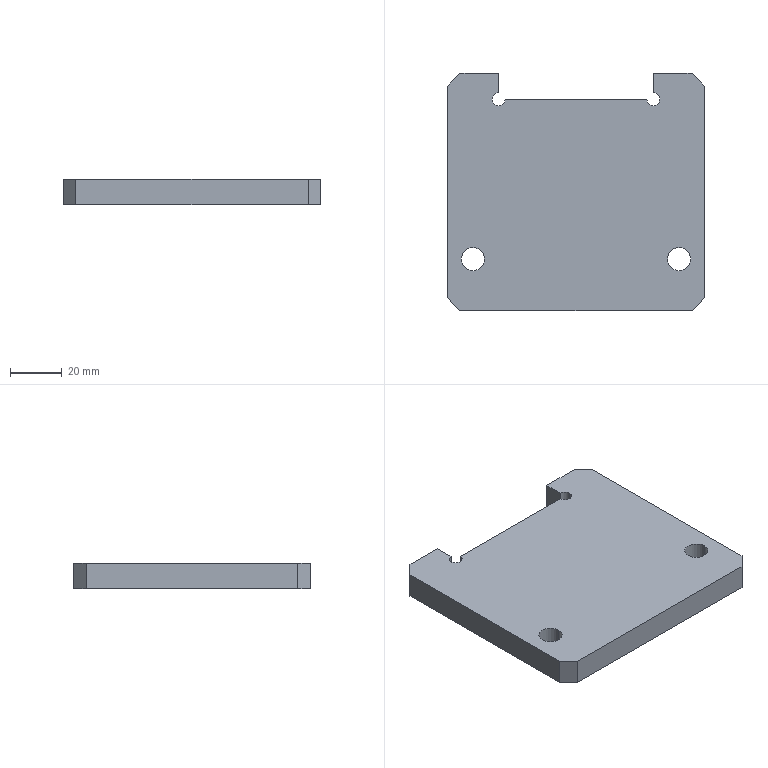Part | SolidWorks | features BaseBody 1 | 1 solid | 29 faces | box 100 x 92 x 10 mm | volume 83534 mm3 | plane 14 | cylinder 11 | cone 4 | commonest cylinder face diameters 4.2 x4 9 x4 5 x3
STEP:
#1=CARTESIAN_POINT('',(35.5,-26.,0.));
#2=VERTEX_POINT('',#1);
#3=CARTESIAN_POINT('',(44.5,-26.,0.));
#4=VERTEX_POINT('',#3);
#5=CARTESIAN_POINT('',(40.,-26.,0.));
#6=DIRECTION('',(0.,0.,1.));
#7=DIRECTION('',(1.,0.,0.));
#8=AXIS2_PLACEMENT_3D('',#5,#6,#7);
#9=CIRCLE('',#8,4.5);
#10=EDGE_CURVE('',#2,#4,#9,.T.);
#11=ORIENTED_EDGE('',*,*,#10,.F.);
#12=CARTESIAN_POINT('',(35.5,-26.,10.));
#13=VERTEX_POINT('',#12);
#14=CARTESIAN_POINT('',(35.5,-26.,10.));
#15=DIRECTION('',(0.,0.,1.));
#16=VECTOR('',#15,1000.);
#17=LINE('',#14,#16);
#18=EDGE_CURVE('',#2,#13,#17,.T.);
#19=ORIENTED_EDGE('',*,*,#18,.T.);
#20=CARTESIAN_POINT('',(44.5,-26.,10.));
#21=VERTEX_POINT('',#20);
#22=CARTESIAN_POINT('',(40.,-26.,10.));
#23=DIRECTION('',(0.,0.,1.));
#24=DIRECTION('',(1.,0.,0.));
#25=AXIS2_PLACEMENT_3D('',#22,#23,#24);
#26=CIRCLE('',#25,4.5);
#27=EDGE_CURVE('',#13,#21,#26,.T.);
#28=ORIENTED_EDGE('',*,*,#27,.T.);
#29=CARTESIAN_POINT('',(44.5,-26.,10.));
#30=DIRECTION('',(0.,0.,1.));
#31=VECTOR('',#30,1000.);
#32=LINE('',#29,#31);
#33=EDGE_CURVE('',#4,#21,#32,.T.);
#34=ORIENTED_EDGE('',*,*,#33,.F.);
#35=EDGE_LOOP('',(#11,#19,#28,#34));
#36=FACE_OUTER_BOUND('',#35,.T.);
#37=CARTESIAN_POINT('',(40.,-26.,10.));
#38=DIRECTION('',(0.,0.,1.));
#39=DIRECTION('',(1.,0.,0.));
#40=AXIS2_PLACEMENT_3D('',#37,#38,#39);
#41=CYLINDRICAL_SURFACE('',#40,4.5);
#42=ADVANCED_FACE('',(#36),#41,.F.);
#43=CARTESIAN_POINT('',(-44.5,-26.,0.));
#44=VERTEX_POINT('',#43);
#45=CARTESIAN_POINT('',(-35.5,-26.,0.));
#46=VERTEX_POINT('',#45);
#47=CARTESIAN_POINT('',(-40.,-26.,0.));
#48=DIRECTION('',(0.,0.,1.));
#49=DIRECTION('',(1.,0.,0.));
#50=AXIS2_PLACEMENT_3D('',#47,#48,#49);
#51=CIRCLE('',#50,4.5);
#52=EDGE_CURVE('',#44,#46,#51,.T.);
#53=ORIENTED_EDGE('',*,*,#52,.F.);
#54=CARTESIAN_POINT('',(-44.5,-26.,10.));
#55=VERTEX_POINT('',#54);
#56=CARTESIAN_POINT('',(-44.5,-26.,10.));
#57=DIRECTION('',(0.,0.,1.));
#58=VECTOR('',#57,1000.);
#59=LINE('',#56,#58);
#60=EDGE_CURVE('',#44,#55,#59,.T.);
#61=ORIENTED_EDGE('',*,*,#60,.T.);
#62=CARTESIAN_POINT('',(-35.5,-26.,10.));
#63=VERTEX_POINT('',#62);
#64=CARTESIAN_POINT('',(-40.,-26.,10.));
#65=DIRECTION('',(0.,0.,1.));
#66=DIRECTION('',(1.,0.,0.));
#67=AXIS2_PLACEMENT_3D('',#64,#65,#66);
#68=CIRCLE('',#67,4.5);
#69=EDGE_CURVE('',#55,#63,#68,.T.);
#70=ORIENTED_EDGE('',*,*,#69,.T.);
#71=CARTESIAN_POINT('',(-35.5,-26.,10.));
#72=DIRECTION('',(0.,0.,1.));
#73=VECTOR('',#72,1000.);
#74=LINE('',#71,#73);
#75=EDGE_CURVE('',#46,#63,#74,.T.);
#76=ORIENTED_EDGE('',*,*,#75,.F.);
#77=EDGE_LOOP('',(#53,#61,#70,#76));
#78=FACE_OUTER_BOUND('',#77,.T.);
#79=CARTESIAN_POINT('',(-40.,-26.,10.));
#80=DIRECTION('',(0.,0.,1.));
#81=DIRECTION('',(1.,0.,0.));
#82=AXIS2_PLACEMENT_3D('',#79,#80,#81);
#83=CYLINDRICAL_SURFACE('',#82,4.5);
#84=ADVANCED_FACE('',(#78),#83,.F.);
#85=CARTESIAN_POINT('',(-20.,22.,2.9));
#86=VERTEX_POINT('',#85);
#87=CARTESIAN_POINT('',(-20.,22.,7.1));
#88=VERTEX_POINT('',#87);
#89=CARTESIAN_POINT('',(-20.,22.,5.));
#90=DIRECTION('',(0.,1.,0.));
#91=DIRECTION('',(0.,0.,1.));
#92=AXIS2_PLACEMENT_3D('',#89,#90,#91);
#93=CIRCLE('',#92,2.1);
#94=EDGE_CURVE('',#86,#88,#93,.T.);
#95=ORIENTED_EDGE('',*,*,#94,.F.);
#96=CARTESIAN_POINT('',(-20.,36.,2.9));
#97=VERTEX_POINT('',#96);
#98=CARTESIAN_POINT('',(-20.,36.,2.9));
#99=DIRECTION('',(0.,1.,0.));
#100=VECTOR('',#99,1000.);
#101=LINE('',#98,#100);
#102=EDGE_CURVE('',#86,#97,#101,.T.);
#103=ORIENTED_EDGE('',*,*,#102,.T.);
#104=CARTESIAN_POINT('',(-20.,36.,7.1));
#105=VERTEX_POINT('',#104);
#106=CARTESIAN_POINT('',(-20.,36.,5.));
#107=DIRECTION('',(0.,1.,0.));
#108=DIRECTION('',(0.,0.,1.));
#109=AXIS2_PLACEMENT_3D('',#106,#107,#108);
#110=CIRCLE('',#109,2.1);
#111=EDGE_CURVE('',#97,#105,#110,.T.);
#112=ORIENTED_EDGE('',*,*,#111,.T.);
#113=CARTESIAN_POINT('',(-20.,36.,7.1));
#114=DIRECTION('',(0.,1.,0.));
#115=VECTOR('',#114,1000.);
#116=LINE('',#113,#115);
#117=EDGE_CURVE('',#88,#105,#116,.T.);
#118=ORIENTED_EDGE('',*,*,#117,.F.);
#119=EDGE_LOOP('',(#95,#103,#112,#118));
#120=FACE_OUTER_BOUND('',#119,.T.);
#121=CARTESIAN_POINT('',(-20.,36.,5.));
#122=DIRECTION('',(0.,1.,0.));
#123=DIRECTION('',(0.,0.,1.));
#124=AXIS2_PLACEMENT_3D('',#121,#122,#123);
#125=CYLINDRICAL_SURFACE('',#124,2.1);
#126=ADVANCED_FACE('',(#120),#125,.F.);
#127=CARTESIAN_POINT('',(-20.,20.738,5.));
#128=VERTEX_POINT('',#127);
#129=CARTESIAN_POINT('',(-20.,22.,7.1));
#130=DIRECTION('',(0.,0.515,0.8572));
#131=VECTOR('',#130,1000.);
#132=LINE('',#129,#131);
#133=EDGE_CURVE('',#128,#88,#132,.T.);
#134=ORIENTED_EDGE('',*,*,#133,.F.);
#135=CARTESIAN_POINT('',(-20.,22.,2.9));
#136=DIRECTION('',(0.,0.515,-0.8572));
#137=VECTOR('',#136,1000.);
#138=LINE('',#135,#137);
#139=EDGE_CURVE('',#128,#86,#138,.T.);
#140=ORIENTED_EDGE('',*,*,#139,.T.);
#141=ORIENTED_EDGE('',*,*,#94,.T.);
#142=EDGE_LOOP('',(#134,#140,#141));
#143=FACE_OUTER_BOUND('',#142,.T.);
#144=CARTESIAN_POINT('',(-20.,22.,5.));
#145=DIRECTION('',(0.,1.,0.));
#146=DIRECTION('',(0.,0.,1.));
#147=AXIS2_PLACEMENT_3D('',#144,#145,#146);
#148=CONICAL_SURFACE('',#147,2.1,1.03);
#149=ADVANCED_FACE('',(#143),#148,.F.);
#150=CARTESIAN_POINT('',(20.,22.,2.9));
#151=VERTEX_POINT('',#150);
#152=CARTESIAN_POINT('',(20.,22.,7.1));
#153=VERTEX_POINT('',#152);
#154=CARTESIAN_POINT('',(20.,22.,5.));
#155=DIRECTION('',(0.,1.,0.));
#156=DIRECTION('',(0.,0.,1.));
#157=AXIS2_PLACEMENT_3D('',#154,#155,#156);
#158=CIRCLE('',#157,2.1);
#159=EDGE_CURVE('',#151,#153,#158,.T.);
#160=ORIENTED_EDGE('',*,*,#159,.F.);
#161=CARTESIAN_POINT('',(20.,36.,2.9));
#162=VERTEX_POINT('',#161);
#163=CARTESIAN_POINT('',(20.,36.,2.9));
#164=DIRECTION('',(0.,1.,0.));
#165=VECTOR('',#164,1000.);
#166=LINE('',#163,#165);
#167=EDGE_CURVE('',#151,#162,#166,.T.);
#168=ORIENTED_EDGE('',*,*,#167,.T.);
#169=CARTESIAN_POINT('',(20.,36.,7.1));
#170=VERTEX_POINT('',#169);
#171=CARTESIAN_POINT('',(20.,36.,5.));
#172=DIRECTION('',(0.,1.,0.));
#173=DIRECTION('',(0.,0.,1.));
#174=AXIS2_PLACEMENT_3D('',#171,#172,#173);
#175=CIRCLE('',#174,2.1);
#176=EDGE_CURVE('',#162,#170,#175,.T.);
#177=ORIENTED_EDGE('',*,*,#176,.T.);
#178=CARTESIAN_POINT('',(20.,36.,7.1));
#179=DIRECTION('',(0.,1.,0.));
#180=VECTOR('',#179,1000.);
#181=LINE('',#178,#180);
#182=EDGE_CURVE('',#153,#170,#181,.T.);
#183=ORIENTED_EDGE('',*,*,#182,.F.);
#184=EDGE_LOOP('',(#160,#168,#177,#183));
#185=FACE_OUTER_BOUND('',#184,.T.);
#186=CARTESIAN_POINT('',(20.,36.,5.));
#187=DIRECTION('',(0.,1.,0.));
#188=DIRECTION('',(0.,0.,1.));
#189=AXIS2_PLACEMENT_3D('',#186,#187,#188);
#190=CYLINDRICAL_SURFACE('',#189,2.1);
#191=ADVANCED_FACE('',(#185),#190,.F.);
#192=CARTESIAN_POINT('',(20.,20.738,5.));
#193=VERTEX_POINT('',#192);
#194=CARTESIAN_POINT('',(20.,22.,7.1));
#195=DIRECTION('',(0.,0.515,0.8572));
#196=VECTOR('',#195,1000.);
#197=LINE('',#194,#196);
#198=EDGE_CURVE('',#193,#153,#197,.T.);
#199=ORIENTED_EDGE('',*,*,#198,.F.);
#200=CARTESIAN_POINT('',(20.,22.,2.9));
#201=DIRECTION('',(0.,0.515,-0.8572));
#202=VECTOR('',#201,1000.);
#203=LINE('',#200,#202);
#204=EDGE_CURVE('',#193,#151,#203,.T.);
#205=ORIENTED_EDGE('',*,*,#204,.T.);
#206=ORIENTED_EDGE('',*,*,#159,.T.);
#207=EDGE_LOOP('',(#199,#205,#206));
#208=FACE_OUTER_BOUND('',#207,.T.);
#209=CARTESIAN_POINT('',(20.,22.,5.));
#210=DIRECTION('',(0.,1.,0.));
#211=DIRECTION('',(0.,0.,1.));
#212=AXIS2_PLACEMENT_3D('',#209,#210,#211);
#213=CONICAL_SURFACE('',#212,2.1,1.03);
#214=ADVANCED_FACE('',(#208),#213,.F.);
#215=CARTESIAN_POINT('',(32.5,36.,0.));
#216=VERTEX_POINT('',#215);
#217=CARTESIAN_POINT('',(30.,38.5,0.));
#218=VERTEX_POINT('',#217);
#219=CARTESIAN_POINT('',(30.,36.,0.));
#220=DIRECTION('',(0.,0.,1.));
#221=DIRECTION('',(1.,0.,0.));
#222=AXIS2_PLACEMENT_3D('',#219,#220,#221);
#223=CIRCLE('',#222,2.5);
#224=EDGE_CURVE('',#216,#218,#223,.T.);
#225=ORIENTED_EDGE('',*,*,#224,.F.);
#226=CARTESIAN_POINT('',(32.5,36.,10.));
#227=VERTEX_POINT('',#226);
#228=CARTESIAN_POINT('',(32.5,36.,0.));
#229=DIRECTION('',(0.,0.,1.));
#230=VECTOR('',#229,1000.);
#231=LINE('',#228,#230);
#232=EDGE_CURVE('',#216,#227,#231,.T.);
#233=ORIENTED_EDGE('',*,*,#232,.T.);
#234=CARTESIAN_POINT('',(30.,38.5,10.));
#235=VERTEX_POINT('',#234);
#236=CARTESIAN_POINT('',(30.,36.,10.));
#237=DIRECTION('',(0.,0.,1.));
#238=DIRECTION('',(1.,0.,0.));
#239=AXIS2_PLACEMENT_3D('',#236,#237,#238);
#240=CIRCLE('',#239,2.5);
#241=EDGE_CURVE('',#227,#235,#240,.T.);
#242=ORIENTED_EDGE('',*,*,#241,.T.);
#243=CARTESIAN_POINT('',(30.,38.5,0.));
#244=DIRECTION('',(0.,0.,1.));
#245=VECTOR('',#244,1000.);
#246=LINE('',#243,#245);
#247=EDGE_CURVE('',#218,#235,#246,.T.);
#248=ORIENTED_EDGE('',*,*,#247,.F.);
#249=EDGE_LOOP('',(#225,#233,#242,#248));
#250=FACE_OUTER_BOUND('',#249,.T.);
#251=CARTESIAN_POINT('',(30.,36.,0.));
#252=DIRECTION('',(0.,0.,1.));
#253=DIRECTION('',(1.,0.,0.));
#254=AXIS2_PLACEMENT_3D('',#251,#252,#253);
#255=CYLINDRICAL_SURFACE('',#254,2.5);
#256=ADVANCED_FACE('',(#250),#255,.F.);
#257=CARTESIAN_POINT('',(-30.,46.,0.));
#258=VERTEX_POINT('',#257);
#259=CARTESIAN_POINT('',(-45.,46.,0.));
#260=VERTEX_POINT('',#259);
#261=CARTESIAN_POINT('',(50.,46.,0.));
#262=DIRECTION('',(-1.,0.,0.));
#263=VECTOR('',#262,1000.);
#264=LINE('',#261,#263);
#265=EDGE_CURVE('',#258,#260,#264,.T.);
#266=ORIENTED_EDGE('',*,*,#265,.T.);
#267=CARTESIAN_POINT('',(-45.,46.,10.));
#268=VERTEX_POINT('',#267);
#269=CARTESIAN_POINT('',(-45.,46.,10.));
#270=DIRECTION('',(0.,0.,1.));
#271=VECTOR('',#270,1000.);
#272=LINE('',#269,#271);
#273=EDGE_CURVE('',#260,#268,#272,.T.);
#274=ORIENTED_EDGE('',*,*,#273,.T.);
#275=CARTESIAN_POINT('',(-30.,46.,10.));
#276=VERTEX_POINT('',#275);
#277=CARTESIAN_POINT('',(50.,46.,10.));
#278=DIRECTION('',(-1.,0.,0.));
#279=VECTOR('',#278,1000.);
#280=LINE('',#277,#279);
#281=EDGE_CURVE('',#276,#268,#280,.T.);
#282=ORIENTED_EDGE('',*,*,#281,.F.);
#283=CARTESIAN_POINT('',(-30.,46.,10.));
#284=DIRECTION('',(0.,0.,-1.));
#285=VECTOR('',#284,1000.);
#286=LINE('',#283,#285);
#287=EDGE_CURVE('',#276,#258,#286,.T.);
#288=ORIENTED_EDGE('',*,*,#287,.T.);
#289=EDGE_LOOP('',(#266,#274,#282,#288));
#290=FACE_OUTER_BOUND('',#289,.T.);
#291=CARTESIAN_POINT('',(50.,46.,10.));
#292=DIRECTION('',(0.,-1.,0.));
#293=DIRECTION('',(1.,0.,0.));
#294=AXIS2_PLACEMENT_3D('',#291,#292,#293);
#295=PLANE('',#294);
#296=ADVANCED_FACE('',(#290),#295,.F.);
#297=CARTESIAN_POINT('',(-50.,41.,0.));
#298=VERTEX_POINT('',#297);
#299=CARTESIAN_POINT('',(-50.,-41.,0.));
#300=VERTEX_POINT('',#299);
#301=CARTESIAN_POINT('',(-50.,-46.,0.));
#302=DIRECTION('',(0.,-1.,0.));
#303=VECTOR('',#302,1000.);
#304=LINE('',#301,#303);
#305=EDGE_CURVE('',#298,#300,#304,.T.);
#306=ORIENTED_EDGE('',*,*,#305,.T.);
#307=CARTESIAN_POINT('',(-50.,-41.,10.));
#308=VERTEX_POINT('',#307);
#309=CARTESIAN_POINT('',(-50.,-41.,10.));
#310=DIRECTION('',(0.,0.,1.));
#311=VECTOR('',#310,1000.);
#312=LINE('',#309,#311);
#313=EDGE_CURVE('',#300,#308,#312,.T.);
#314=ORIENTED_EDGE('',*,*,#313,.T.);
#315=CARTESIAN_POINT('',(-50.,41.,10.));
#316=VERTEX_POINT('',#315);
#317=CARTESIAN_POINT('',(-50.,-46.,10.));
#318=DIRECTION('',(0.,-1.,0.));
#319=VECTOR('',#318,1000.);
#320=LINE('',#317,#319);
#321=EDGE_CURVE('',#316,#308,#320,.T.);
#322=ORIENTED_EDGE('',*,*,#321,.F.);
#323=CARTESIAN_POINT('',(-50.,41.,10.));
#324=DIRECTION('',(0.,0.,-1.));
#325=VECTOR('',#324,1000.);
#326=LINE('',#323,#325);
#327=EDGE_CURVE('',#316,#298,#326,.T.);
#328=ORIENTED_EDGE('',*,*,#327,.T.);
#329=EDGE_LOOP('',(#306,#314,#322,#328));
#330=FACE_OUTER_BOUND('',#329,.T.);
#331=CARTESIAN_POINT('',(-50.,-46.,10.));
#332=DIRECTION('',(1.,0.,0.));
#333=DIRECTION('',(0.,0.,-1.));
#334=AXIS2_PLACEMENT_3D('',#331,#332,#333);
#335=PLANE('',#334);
#336=ADVANCED_FACE('',(#330),#335,.F.);
#337=CARTESIAN_POINT('',(-45.,-46.,10.));
#338=VERTEX_POINT('',#337);
#339=CARTESIAN_POINT('',(45.,-46.,10.));
#340=VERTEX_POINT('',#339);
#341=CARTESIAN_POINT('',(50.,-46.,10.));
#342=DIRECTION('',(1.,0.,0.));
#343=VECTOR('',#342,1000.);
#344=LINE('',#341,#343);
#345=EDGE_CURVE('',#338,#340,#344,.T.);
#346=ORIENTED_EDGE('',*,*,#345,.F.);
#347=CARTESIAN_POINT('',(-45.,-46.,0.));
#348=VERTEX_POINT('',#347);
#349=CARTESIAN_POINT('',(-45.,-46.,10.));
#350=DIRECTION('',(0.,0.,-1.));
#351=VECTOR('',#350,1000.);
#352=LINE('',#349,#351);
#353=EDGE_CURVE('',#338,#348,#352,.T.);
#354=ORIENTED_EDGE('',*,*,#353,.T.);
#355=CARTESIAN_POINT('',(45.,-46.,0.));
#356=VERTEX_POINT('',#355);
#357=CARTESIAN_POINT('',(50.,-46.,0.));
#358=DIRECTION('',(1.,0.,0.));
#359=VECTOR('',#358,1000.);
#360=LINE('',#357,#359);
#361=EDGE_CURVE('',#348,#356,#360,.T.);
#362=ORIENTED_EDGE('',*,*,#361,.T.);
#363=CARTESIAN_POINT('',(45.,-46.,10.));
#364=DIRECTION('',(0.,0.,1.));
#365=VECTOR('',#364,1000.);
#366=LINE('',#363,#365);
#367=EDGE_CURVE('',#356,#340,#366,.T.);
#368=ORIENTED_EDGE('',*,*,#367,.T.);
#369=EDGE_LOOP('',(#346,#354,#362,#368));
#370=FACE_OUTER_BOUND('',#369,.T.);
#371=CARTESIAN_POINT('',(50.,-46.,10.));
#372=DIRECTION('',(0.,1.,0.));
#373=DIRECTION('',(-1.,0.,0.));
#374=AXIS2_PLACEMENT_3D('',#371,#372,#373);
#375=PLANE('',#374);
#376=ADVANCED_FACE('',(#370),#375,.F.);
#377=CARTESIAN_POINT('',(50.,-41.,10.));
#378=VERTEX_POINT('',#377);
#379=CARTESIAN_POINT('',(50.,41.,10.));
#380=VERTEX_POINT('',#379);
#381=CARTESIAN_POINT('',(50.,-46.,10.));
#382=DIRECTION('',(0.,1.,0.));
#383=VECTOR('',#382,1000.);
#384=LINE('',#381,#383);
#385=EDGE_CURVE('',#378,#380,#384,.T.);
#386=ORIENTED_EDGE('',*,*,#385,.F.);
#387=CARTESIAN_POINT('',(50.,-41.,0.));
#388=VERTEX_POINT('',#387);
#389=CARTESIAN_POINT('',(50.,-41.,10.));
#390=DIRECTION('',(0.,0.,-1.));
#391=VECTOR('',#390,1000.);
#392=LINE('',#389,#391);
#393=EDGE_CURVE('',#378,#388,#392,.T.);
#394=ORIENTED_EDGE('',*,*,#393,.T.);
#395=CARTESIAN_POINT('',(50.,41.,0.));
#396=VERTEX_POINT('',#395);
#397=CARTESIAN_POINT('',(50.,-46.,0.));
#398=DIRECTION('',(0.,1.,0.));
#399=VECTOR('',#398,1000.);
#400=LINE('',#397,#399);
#401=EDGE_CURVE('',#388,#396,#400,.T.);
#402=ORIENTED_EDGE('',*,*,#401,.T.);
#403=CARTESIAN_POINT('',(50.,41.,10.));
#404=DIRECTION('',(0.,0.,1.));
#405=VECTOR('',#404,1000.);
#406=LINE('',#403,#405);
#407=EDGE_CURVE('',#396,#380,#406,.T.);
#408=ORIENTED_EDGE('',*,*,#407,.T.);
#409=EDGE_LOOP('',(#386,#394,#402,#408));
#410=FACE_OUTER_BOUND('',#409,.T.);
#411=CARTESIAN_POINT('',(50.,-46.,10.));
#412=DIRECTION('',(-1.,0.,0.));
#413=DIRECTION('',(0.,0.,1.));
#414=AXIS2_PLACEMENT_3D('',#411,#412,#413);
#415=PLANE('',#414);
#416=ADVANCED_FACE('',(#410),#415,.F.);
#417=CARTESIAN_POINT('',(45.,46.,10.));
#418=VERTEX_POINT('',#417);
#419=CARTESIAN_POINT('',(30.,46.,10.));
#420=VERTEX_POINT('',#419);
#421=CARTESIAN_POINT('',(50.,46.,10.));
#422=DIRECTION('',(-1.,0.,0.));
#423=VECTOR('',#422,1000.);
#424=LINE('',#421,#423);
#425=EDGE_CURVE('',#418,#420,#424,.T.);
#426=ORIENTED_EDGE('',*,*,#425,.F.);
#427=CARTESIAN_POINT('',(45.,46.,0.));
#428=VERTEX_POINT('',#427);
#429=CARTESIAN_POINT('',(45.,46.,10.));
#430=DIRECTION('',(0.,0.,-1.));
#431=VECTOR('',#430,1000.);
#432=LINE('',#429,#431);
#433=EDGE_CURVE('',#418,#428,#432,.T.);
#434=ORIENTED_EDGE('',*,*,#433,.T.);
#435=CARTESIAN_POINT('',(30.,46.,0.));
#436=VERTEX_POINT('',#435);
#437=CARTESIAN_POINT('',(50.,46.,0.));
#438=DIRECTION('',(-1.,0.,0.));
#439=VECTOR('',#438,1000.);
#440=LINE('',#437,#439);
#441=EDGE_CURVE('',#428,#436,#440,.T.);
#442=ORIENTED_EDGE('',*,*,#441,.T.);
#443=CARTESIAN_POINT('',(30.,46.,10.));
#444=DIRECTION('',(0.,0.,1.));
#445=VECTOR('',#444,1000.);
#446=LINE('',#443,#445);
#447=EDGE_CURVE('',#436,#420,#446,.T.);
#448=ORIENTED_EDGE('',*,*,#447,.T.);
#449=EDGE_LOOP('',(#426,#434,#442,#448));
#450=FACE_OUTER_BOUND('',#449,.T.);
#451=CARTESIAN_POINT('',(50.,46.,10.));
#452=DIRECTION('',(0.,-1.,0.));
#453=DIRECTION('',(1.,0.,0.));
#454=AXIS2_PLACEMENT_3D('',#451,#452,#453);
#455=PLANE('',#454);
#456=ADVANCED_FACE('',(#450),#455,.F.);
#457=CARTESIAN_POINT('',(40.,-26.,10.));
#458=DIRECTION('',(0.,0.,1.));
#459=DIRECTION('',(1.,0.,0.));
#460=AXIS2_PLACEMENT_3D('',#457,#458,#459);
#461=CIRCLE('',#460,4.5);
#462=EDGE_CURVE('',#21,#13,#461,.T.);
#463=ORIENTED_EDGE('',*,*,#462,.F.);
#464=ORIENTED_EDGE('',*,*,#27,.F.);
#465=EDGE_LOOP('',(#463,#464));
#466=FACE_BOUND('',#465,.T.);
#467=CARTESIAN_POINT('',(-40.,-26.,10.));
#468=DIRECTION('',(0.,0.,1.));
#469=DIRECTION('',(1.,0.,0.));
#470=AXIS2_PLACEMENT_3D('',#467,#468,#469);
#471=CIRCLE('',#470,4.5);
#472=EDGE_CURVE('',#63,#55,#471,.T.);
#473=ORIENTED_EDGE('',*,*,#472,.F.);
#474=ORIENTED_EDGE('',*,*,#69,.F.);
#475=EDGE_LOOP('',(#473,#474));
#476=FACE_BOUND('',#475,.T.);
#477=CARTESIAN_POINT('',(27.5,36.,10.));
#478=VERTEX_POINT('',#477);
#479=CARTESIAN_POINT('',(30.,36.,10.));
#480=DIRECTION('',(0.,0.,1.));
#481=DIRECTION('',(1.,0.,0.));
#482=AXIS2_PLACEMENT_3D('',#479,#480,#481);
#483=CIRCLE('',#482,2.5);
#484=EDGE_CURVE('',#478,#227,#483,.T.);
#485=ORIENTED_EDGE('',*,*,#484,.F.);
#486=CARTESIAN_POINT('',(-27.5,36.,10.));
#487=VERTEX_POINT('',#486);
#488=CARTESIAN_POINT('',(30.,36.,10.));
#489=DIRECTION('',(1.,0.,0.));
#490=VECTOR('',#489,1000.);
#491=LINE('',#488,#490);
#492=EDGE_CURVE('',#487,#478,#491,.T.);
#493=ORIENTED_EDGE('',*,*,#492,.F.);
#494=CARTESIAN_POINT('',(-30.,38.5,10.));
#495=VERTEX_POINT('',#494);
#496=CARTESIAN_POINT('',(-30.,36.,10.));
#497=DIRECTION('',(0.,0.,1.));
#498=DIRECTION('',(1.,0.,0.));
#499=AXIS2_PLACEMENT_3D('',#496,#497,#498);
#500=CIRCLE('',#499,2.5);
#501=EDGE_CURVE('',#495,#487,#500,.T.);
#502=ORIENTED_EDGE('',*,*,#501,.F.);
#503=CARTESIAN_POINT('',(-30.,56.,10.));
#504=DIRECTION('',(0.,-1.,0.));
#505=VECTOR('',#504,1000.);
#506=LINE('',#503,#505);
#507=EDGE_CURVE('',#276,#495,#506,.T.);
#508=ORIENTED_EDGE('',*,*,#507,.F.);
#509=ORIENTED_EDGE('',*,*,#281,.T.);
#510=CARTESIAN_POINT('',(-45.5,45.5,10.));
#511=DIRECTION('',(-0.7071,-0.7071,0.));
#512=VECTOR('',#511,1000.);
#513=LINE('',#510,#512);
#514=EDGE_CURVE('',#268,#316,#513,.T.);
#515=ORIENTED_EDGE('',*,*,#514,.T.);
#516=ORIENTED_EDGE('',*,*,#321,.T.);
#517=CARTESIAN_POINT('',(-45.5,-45.5,10.));
#518=DIRECTION('',(0.7071,-0.7071,0.));
#519=VECTOR('',#518,1000.);
#520=LINE('',#517,#519);
#521=EDGE_CURVE('',#308,#338,#520,.T.);
#522=ORIENTED_EDGE('',*,*,#521,.T.);
#523=ORIENTED_EDGE('',*,*,#345,.T.);
#524=CARTESIAN_POINT('',(45.5,-45.5,10.));
#525=DIRECTION('',(0.7071,0.7071,0.));
#526=VECTOR('',#525,1000.);
#527=LINE('',#524,#526);
#528=EDGE_CURVE('',#340,#378,#527,.T.);
#529=ORIENTED_EDGE('',*,*,#528,.T.);
#530=ORIENTED_EDGE('',*,*,#385,.T.);
#531=CARTESIAN_POINT('',(45.5,45.5,10.));
#532=DIRECTION('',(-0.7071,0.7071,0.));
#533=VECTOR('',#532,1000.);
#534=LINE('',#531,#533);
#535=EDGE_CURVE('',#380,#418,#534,.T.);
#536=ORIENTED_EDGE('',*,*,#535,.T.);
#537=ORIENTED_EDGE('',*,*,#425,.T.);
#538=CARTESIAN_POINT('',(30.,56.,10.));
#539=DIRECTION('',(0.,1.,0.));
#540=VECTOR('',#539,1000.);
#541=LINE('',#538,#540);
#542=EDGE_CURVE('',#235,#420,#541,.T.);
#543=ORIENTED_EDGE('',*,*,#542,.F.);
#544=ORIENTED_EDGE('',*,*,#241,.F.);
#545=EDGE_LOOP('',(#485,#493,#502,#508,#509,#515,#516,#522,#523,#529,#530,#536,#537,#543,#544));
#546=FACE_OUTER_BOUND('',#545,.T.);
#547=CARTESIAN_POINT('',(0.,0.,10.));
#548=DIRECTION('',(0.,0.,1.));
#549=DIRECTION('',(1.,0.,0.));
#550=AXIS2_PLACEMENT_3D('',#547,#548,#549);
#551=PLANE('',#550);
#552=ADVANCED_FACE('',(#466,#476,#546),#551,.T.);
#553=CARTESIAN_POINT('',(40.,-26.,0.));
#554=DIRECTION('',(0.,0.,1.));
#555=DIRECTION('',(1.,0.,0.));
#556=AXIS2_PLACEMENT_3D('',#553,#554,#555);
#557=CIRCLE('',#556,4.5);
#558=EDGE_CURVE('',#4,#2,#557,.T.);
#559=ORIENTED_EDGE('',*,*,#558,.T.);
#560=ORIENTED_EDGE('',*,*,#10,.T.);
#561=EDGE_LOOP('',(#559,#560));
#562=FACE_BOUND('',#561,.T.);
#563=CARTESIAN_POINT('',(-40.,-26.,0.));
#564=DIRECTION('',(0.,0.,1.));
#565=DIRECTION('',(1.,0.,0.));
#566=AXIS2_PLACEMENT_3D('',#563,#564,#565);
#567=CIRCLE('',#566,4.5);
#568=EDGE_CURVE('',#46,#44,#567,.T.);
#569=ORIENTED_EDGE('',*,*,#568,.T.);
#570=ORIENTED_EDGE('',*,*,#52,.T.);
#571=EDGE_LOOP('',(#569,#570));
#572=FACE_BOUND('',#571,.T.);
#573=CARTESIAN_POINT('',(-27.5,36.,0.));
#574=VERTEX_POINT('',#573);
#575=CARTESIAN_POINT('',(27.5,36.,0.));
#576=VERTEX_POINT('',#575);
#577=CARTESIAN_POINT('',(30.,36.,0.));
#578=DIRECTION('',(1.,0.,0.));
#579=VECTOR('',#578,1000.);
#580=LINE('',#577,#579);
#581=EDGE_CURVE('',#574,#576,#580,.T.);
#582=ORIENTED_EDGE('',*,*,#581,.T.);
#583=CARTESIAN_POINT('',(30.,36.,0.));
#584=DIRECTION('',(0.,0.,1.));
#585=DIRECTION('',(1.,0.,0.));
#586=AXIS2_PLACEMENT_3D('',#583,#584,#585);
#587=CIRCLE('',#586,2.5);
#588=EDGE_CURVE('',#576,#216,#587,.T.);
#589=ORIENTED_EDGE('',*,*,#588,.T.);
#590=ORIENTED_EDGE('',*,*,#224,.T.);
#591=CARTESIAN_POINT('',(30.,56.,0.));
#592=DIRECTION('',(0.,1.,0.));
#593=VECTOR('',#592,1000.);
#594=LINE('',#591,#593);
#595=EDGE_CURVE('',#218,#436,#594,.T.);
#596=ORIENTED_EDGE('',*,*,#595,.T.);
#597=ORIENTED_EDGE('',*,*,#441,.F.);
#598=CARTESIAN_POINT('',(45.,46.,0.));
#599=DIRECTION('',(0.7071,-0.7071,0.));
#600=VECTOR('',#599,1000.);
#601=LINE('',#598,#600);
#602=EDGE_CURVE('',#428,#396,#601,.T.);
#603=ORIENTED_EDGE('',*,*,#602,.T.);
#604=ORIENTED_EDGE('',*,*,#401,.F.);
#605=CARTESIAN_POINT('',(50.,-41.,0.));
#606=DIRECTION('',(-0.7071,-0.7071,0.));
#607=VECTOR('',#606,1000.);
#608=LINE('',#605,#607);
#609=EDGE_CURVE('',#388,#356,#608,.T.);
#610=ORIENTED_EDGE('',*,*,#609,.T.);
#611=ORIENTED_EDGE('',*,*,#361,.F.);
#612=CARTESIAN_POINT('',(-45.,-46.,0.));
#613=DIRECTION('',(-0.7071,0.7071,0.));
#614=VECTOR('',#613,1000.);
#615=LINE('',#612,#614);
#616=EDGE_CURVE('',#348,#300,#615,.T.);
#617=ORIENTED_EDGE('',*,*,#616,.T.);
#618=ORIENTED_EDGE('',*,*,#305,.F.);
#619=CARTESIAN_POINT('',(-50.,41.,0.));
#620=DIRECTION('',(0.7071,0.7071,0.));
#621=VECTOR('',#620,1000.);
#622=LINE('',#619,#621);
#623=EDGE_CURVE('',#298,#260,#622,.T.);
#624=ORIENTED_EDGE('',*,*,#623,.T.);
#625=ORIENTED_EDGE('',*,*,#265,.F.);
#626=CARTESIAN_POINT('',(-30.,38.5,0.));
#627=VERTEX_POINT('',#626);
#628=CARTESIAN_POINT('',(-30.,0.,0.));
#629=DIRECTION('',(0.,-1.,0.));
#630=VECTOR('',#629,1000.);
#631=LINE('',#628,#630);
#632=EDGE_CURVE('',#258,#627,#631,.T.);
#633=ORIENTED_EDGE('',*,*,#632,.T.);
#634=CARTESIAN_POINT('',(-30.,36.,0.));
#635=DIRECTION('',(0.,0.,1.));
#636=DIRECTION('',(1.,0.,0.));
#637=AXIS2_PLACEMENT_3D('',#634,#635,#636);
#638=CIRCLE('',#637,2.5);
#639=EDGE_CURVE('',#627,#574,#638,.T.);
#640=ORIENTED_EDGE('',*,*,#639,.T.);
#641=EDGE_LOOP('',(#582,#589,#590,#596,#597,#603,#604,#610,#611,#617,#618,#624,#625,#633,#640));
#642=FACE_OUTER_BOUND('',#641,.T.);
#643=CARTESIAN_POINT('',(0.,0.,0.));
#644=DIRECTION('',(0.,0.,1.));
#645=DIRECTION('',(1.,0.,0.));
#646=AXIS2_PLACEMENT_3D('',#643,#644,#645);
#647=PLANE('',#646);
#648=ADVANCED_FACE('',(#562,#572,#642),#647,.F.);
#649=ORIENTED_EDGE('',*,*,#507,.T.);
#650=CARTESIAN_POINT('',(-30.,38.5,0.));
#651=DIRECTION('',(0.,0.,-1.));
#652=VECTOR('',#651,1000.);
#653=LINE('',#650,#652);
#654=EDGE_CURVE('',#495,#627,#653,.T.);
#655=ORIENTED_EDGE('',*,*,#654,.T.);
#656=ORIENTED_EDGE('',*,*,#632,.F.);
#657=ORIENTED_EDGE('',*,*,#287,.F.);
#658=EDGE_LOOP('',(#649,#655,#656,#657));
#659=FACE_OUTER_BOUND('',#658,.T.);
#660=CARTESIAN_POINT('',(-30.,56.,0.));
#661=DIRECTION('',(-1.,0.,0.));
#662=DIRECTION('',(0.,0.,1.));
#663=AXIS2_PLACEMENT_3D('',#660,#661,#662);
#664=PLANE('',#663);
#665=ADVANCED_FACE('',(#659),#664,.F.);
#666=ORIENTED_EDGE('',*,*,#595,.F.);
#667=ORIENTED_EDGE('',*,*,#247,.T.);
#668=ORIENTED_EDGE('',*,*,#542,.T.);
#669=ORIENTED_EDGE('',*,*,#447,.F.);
#670=EDGE_LOOP('',(#666,#667,#668,#669));
#671=FACE_OUTER_BOUND('',#670,.T.);
#672=CARTESIAN_POINT('',(30.,56.,0.));
#673=DIRECTION('',(1.,0.,0.));
#674=DIRECTION('',(0.,1.,0.));
#675=AXIS2_PLACEMENT_3D('',#672,#673,#674);
#676=PLANE('',#675);
#677=ADVANCED_FACE('',(#671),#676,.F.);
#678=CARTESIAN_POINT('',(-20.,36.,5.));
#679=DIRECTION('',(0.,1.,0.));
#680=DIRECTION('',(0.,0.,1.));
#681=AXIS2_PLACEMENT_3D('',#678,#679,#680);
#682=CIRCLE('',#681,2.1);
#683=EDGE_CURVE('',#105,#97,#682,.T.);
#684=ORIENTED_EDGE('',*,*,#683,.F.);
#685=ORIENTED_EDGE('',*,*,#111,.F.);
#686=EDGE_LOOP('',(#684,#685));
#687=FACE_BOUND('',#686,.T.);
#688=CARTESIAN_POINT('',(20.,36.,5.));
#689=DIRECTION('',(0.,1.,0.));
#690=DIRECTION('',(0.,0.,1.));
#691=AXIS2_PLACEMENT_3D('',#688,#689,#690);
#692=CIRCLE('',#691,2.1);
#693=EDGE_CURVE('',#170,#162,#692,.T.);
#694=ORIENTED_EDGE('',*,*,#693,.F.);
#695=ORIENTED_EDGE('',*,*,#176,.F.);
#696=EDGE_LOOP('',(#694,#695));
#697=FACE_BOUND('',#696,.T.);
#698=ORIENTED_EDGE('',*,*,#492,.T.);
#699=CARTESIAN_POINT('',(27.5,36.,0.));
#700=DIRECTION('',(0.,0.,-1.));
#701=VECTOR('',#700,1000.);
#702=LINE('',#699,#701);
#703=EDGE_CURVE('',#478,#576,#702,.T.);
#704=ORIENTED_EDGE('',*,*,#703,.T.);
#705=ORIENTED_EDGE('',*,*,#581,.F.);
#706=CARTESIAN_POINT('',(-27.5,36.,0.));
#707=DIRECTION('',(0.,0.,1.));
#708=VECTOR('',#707,1000.);
#709=LINE('',#706,#708);
#710=EDGE_CURVE('',#574,#487,#709,.T.);
#711=ORIENTED_EDGE('',*,*,#710,.T.);
#712=EDGE_LOOP('',(#698,#704,#705,#711));
#713=FACE_OUTER_BOUND('',#712,.T.);
#714=CARTESIAN_POINT('',(30.,36.,0.));
#715=DIRECTION('',(0.,-1.,0.));
#716=DIRECTION('',(0.,0.,-1.));
#717=AXIS2_PLACEMENT_3D('',#714,#715,#716);
#718=PLANE('',#717);
#719=ADVANCED_FACE('',(#687,#697,#713),#718,.F.);
#720=ORIENTED_EDGE('',*,*,#521,.F.);
#721=ORIENTED_EDGE('',*,*,#313,.F.);
#722=ORIENTED_EDGE('',*,*,#616,.F.);
#723=ORIENTED_EDGE('',*,*,#353,.F.);
#724=EDGE_LOOP('',(#720,#721,#722,#723));
#725=FACE_OUTER_BOUND('',#724,.T.);
#726=CARTESIAN_POINT('',(-45.,-46.,10.));
#727=DIRECTION('',(0.7071,0.7071,0.));
#728=DIRECTION('',(0.,0.,-1.));
#729=AXIS2_PLACEMENT_3D('',#726,#727,#728);
#730=PLANE('',#729);
#731=ADVANCED_FACE('',(#725),#730,.F.);
#732=ORIENTED_EDGE('',*,*,#528,.F.);
#733=ORIENTED_EDGE('',*,*,#367,.F.);
#734=ORIENTED_EDGE('',*,*,#609,.F.);
#735=ORIENTED_EDGE('',*,*,#393,.F.);
#736=EDGE_LOOP('',(#732,#733,#734,#735));
#737=FACE_OUTER_BOUND('',#736,.T.);
#738=CARTESIAN_POINT('',(50.,-41.,10.));
#739=DIRECTION('',(-0.7071,0.7071,0.));
#740=DIRECTION('',(0.,0.,-1.));
#741=AXIS2_PLACEMENT_3D('',#738,#739,#740);
#742=PLANE('',#741);
#743=ADVANCED_FACE('',(#737),#742,.F.);
#744=ORIENTED_EDGE('',*,*,#535,.F.);
#745=ORIENTED_EDGE('',*,*,#407,.F.);
#746=ORIENTED_EDGE('',*,*,#602,.F.);
#747=ORIENTED_EDGE('',*,*,#433,.F.);
#748=EDGE_LOOP('',(#744,#745,#746,#747));
#749=FACE_OUTER_BOUND('',#748,.T.);
#750=CARTESIAN_POINT('',(45.,46.,10.));
#751=DIRECTION('',(-0.7071,-0.7071,0.));
#752=DIRECTION('',(0.,0.,-1.));
#753=AXIS2_PLACEMENT_3D('',#750,#751,#752);
#754=PLANE('',#753);
#755=ADVANCED_FACE('',(#749),#754,.F.);
#756=ORIENTED_EDGE('',*,*,#514,.F.);
#757=ORIENTED_EDGE('',*,*,#273,.F.);
#758=ORIENTED_EDGE('',*,*,#623,.F.);
#759=ORIENTED_EDGE('',*,*,#327,.F.);
#760=EDGE_LOOP('',(#756,#757,#758,#759));
#761=FACE_OUTER_BOUND('',#760,.T.);
#762=CARTESIAN_POINT('',(-50.,41.,10.));
#763=DIRECTION('',(0.7071,-0.7071,0.));
#764=DIRECTION('',(0.,0.,-1.));
#765=AXIS2_PLACEMENT_3D('',#762,#763,#764);
#766=PLANE('',#765);
#767=ADVANCED_FACE('',(#761),#766,.F.);
#768=ORIENTED_EDGE('',*,*,#501,.T.);
#769=ORIENTED_EDGE('',*,*,#710,.F.);
#770=ORIENTED_EDGE('',*,*,#639,.F.);
#771=ORIENTED_EDGE('',*,*,#654,.F.);
#772=EDGE_LOOP('',(#768,#769,#770,#771));
#773=FACE_OUTER_BOUND('',#772,.T.);
#774=CARTESIAN_POINT('',(-30.,36.,0.));
#775=DIRECTION('',(0.,0.,1.));
#776=DIRECTION('',(1.,0.,0.));
#777=AXIS2_PLACEMENT_3D('',#774,#775,#776);
#778=CYLINDRICAL_SURFACE('',#777,2.5);
#779=ADVANCED_FACE('',(#773),#778,.F.);
#780=ORIENTED_EDGE('',*,*,#232,.F.);
#781=ORIENTED_EDGE('',*,*,#588,.F.);
#782=ORIENTED_EDGE('',*,*,#703,.F.);
#783=ORIENTED_EDGE('',*,*,#484,.T.);
#784=EDGE_LOOP('',(#780,#781,#782,#783));
#785=FACE_OUTER_BOUND('',#784,.T.);
#786=CARTESIAN_POINT('',(30.,36.,0.));
#787=DIRECTION('',(0.,0.,1.));
#788=DIRECTION('',(1.,0.,0.));
#789=AXIS2_PLACEMENT_3D('',#786,#787,#788);
#790=CYLINDRICAL_SURFACE('',#789,2.5);
#791=ADVANCED_FACE('',(#785),#790,.F.);
#792=ORIENTED_EDGE('',*,*,#204,.F.);
#793=ORIENTED_EDGE('',*,*,#198,.T.);
#794=CARTESIAN_POINT('',(20.,22.,5.));
#795=DIRECTION('',(0.,1.,0.));
#796=DIRECTION('',(0.,0.,1.));
#797=AXIS2_PLACEMENT_3D('',#794,#795,#796);
#798=CIRCLE('',#797,2.1);
#799=EDGE_CURVE('',#153,#151,#798,.T.);
#800=ORIENTED_EDGE('',*,*,#799,.T.);
#801=EDGE_LOOP('',(#792,#793,#800));
#802=FACE_OUTER_BOUND('',#801,.T.);
#803=CARTESIAN_POINT('',(20.,22.,5.));
#804=DIRECTION('',(0.,1.,0.));
#805=DIRECTION('',(0.,0.,1.));
#806=AXIS2_PLACEMENT_3D('',#803,#804,#805);
#807=CONICAL_SURFACE('',#806,2.1,1.03);
#808=ADVANCED_FACE('',(#802),#807,.F.);
#809=ORIENTED_EDGE('',*,*,#167,.F.);
#810=ORIENTED_EDGE('',*,*,#799,.F.);
#811=ORIENTED_EDGE('',*,*,#182,.T.);
#812=ORIENTED_EDGE('',*,*,#693,.T.);
#813=EDGE_LOOP('',(#809,#810,#811,#812));
#814=FACE_OUTER_BOUND('',#813,.T.);
#815=CARTESIAN_POINT('',(20.,36.,5.));
#816=DIRECTION('',(0.,1.,0.));
#817=DIRECTION('',(0.,0.,1.));
#818=AXIS2_PLACEMENT_3D('',#815,#816,#817);
#819=CYLINDRICAL_SURFACE('',#818,2.1);
#820=ADVANCED_FACE('',(#814),#819,.F.);
#821=ORIENTED_EDGE('',*,*,#139,.F.);
#822=ORIENTED_EDGE('',*,*,#133,.T.);
#823=CARTESIAN_POINT('',(-20.,22.,5.));
#824=DIRECTION('',(0.,1.,0.));
#825=DIRECTION('',(0.,0.,1.));
#826=AXIS2_PLACEMENT_3D('',#823,#824,#825);
#827=CIRCLE('',#826,2.1);
#828=EDGE_CURVE('',#88,#86,#827,.T.);
#829=ORIENTED_EDGE('',*,*,#828,.T.);
#830=EDGE_LOOP('',(#821,#822,#829));
#831=FACE_OUTER_BOUND('',#830,.T.);
#832=CARTESIAN_POINT('',(-20.,22.,5.));
#833=DIRECTION('',(0.,1.,0.));
#834=DIRECTION('',(0.,0.,1.));
#835=AXIS2_PLACEMENT_3D('',#832,#833,#834);
#836=CONICAL_SURFACE('',#835,2.1,1.03);
#837=ADVANCED_FACE('',(#831),#836,.F.);
#838=ORIENTED_EDGE('',*,*,#102,.F.);
#839=ORIENTED_EDGE('',*,*,#828,.F.);
#840=ORIENTED_EDGE('',*,*,#117,.T.);
#841=ORIENTED_EDGE('',*,*,#683,.T.);
#842=EDGE_LOOP('',(#838,#839,#840,#841));
#843=FACE_OUTER_BOUND('',#842,.T.);
#844=CARTESIAN_POINT('',(-20.,36.,5.));
#845=DIRECTION('',(0.,1.,0.));
#846=DIRECTION('',(0.,0.,1.));
#847=AXIS2_PLACEMENT_3D('',#844,#845,#846);
#848=CYLINDRICAL_SURFACE('',#847,2.1);
#849=ADVANCED_FACE('',(#843),#848,.F.);
#850=ORIENTED_EDGE('',*,*,#60,.F.);
#851=ORIENTED_EDGE('',*,*,#568,.F.);
#852=ORIENTED_EDGE('',*,*,#75,.T.);
#853=ORIENTED_EDGE('',*,*,#472,.T.);
#854=EDGE_LOOP('',(#850,#851,#852,#853));
#855=FACE_OUTER_BOUND('',#854,.T.);
#856=CARTESIAN_POINT('',(-40.,-26.,10.));
#857=DIRECTION('',(0.,0.,1.));
#858=DIRECTION('',(1.,0.,0.));
#859=AXIS2_PLACEMENT_3D('',#856,#857,#858);
#860=CYLINDRICAL_SURFACE('',#859,4.5);
#861=ADVANCED_FACE('',(#855),#860,.F.);
#862=ORIENTED_EDGE('',*,*,#18,.F.);
#863=ORIENTED_EDGE('',*,*,#558,.F.);
#864=ORIENTED_EDGE('',*,*,#33,.T.);
#865=ORIENTED_EDGE('',*,*,#462,.T.);
#866=EDGE_LOOP('',(#862,#863,#864,#865));
#867=FACE_OUTER_BOUND('',#866,.T.);
#868=CARTESIAN_POINT('',(40.,-26.,10.));
#869=DIRECTION('',(0.,0.,1.));
#870=DIRECTION('',(1.,0.,0.));
#871=AXIS2_PLACEMENT_3D('',#868,#869,#870);
#872=CYLINDRICAL_SURFACE('',#871,4.5);
#873=ADVANCED_FACE('',(#867),#872,.F.);
#874=CLOSED_SHELL('',(#42,#84,#126,#149,#191,#214,#256,#296,#336,#376,#416,#456,#552,#648,#665,#677,#719,#731,#743,#755,#767,#779,#791,#808,#820,#837,#849,#861,#873));
#875=MANIFOLD_SOLID_BREP('',#874);
#876=CARTESIAN_POINT('',(0.,0.,0.));
#877=DIRECTION('',(0.,0.,1.));
#878=DIRECTION('',(1.,0.,0.));
#879=AXIS2_PLACEMENT_3D('',#876,#877,#878);
#880=(LENGTH_UNIT()NAMED_UNIT(*)SI_UNIT(.MILLI.,.METRE.));
#881=UNCERTAINTY_MEASURE_WITH_UNIT(LENGTH_MEASURE(0.00001),#880,'','');
#882=(NAMED_UNIT(*)PLANE_ANGLE_UNIT()SI_UNIT($,.RADIAN.));
#883=(NAMED_UNIT(*)SI_UNIT($,.STERADIAN.)SOLID_ANGLE_UNIT());
#884=(GEOMETRIC_REPRESENTATION_CONTEXT(3)GLOBAL_UNCERTAINTY_ASSIGNED_CONTEXT((#881))GLOBAL_UNIT_ASSIGNED_CONTEXT((#880,#882,#883))REPRESENTATION_CONTEXT('',''));
#885=ADVANCED_BREP_SHAPE_REPRESENTATION('',(#875,#879),#884);